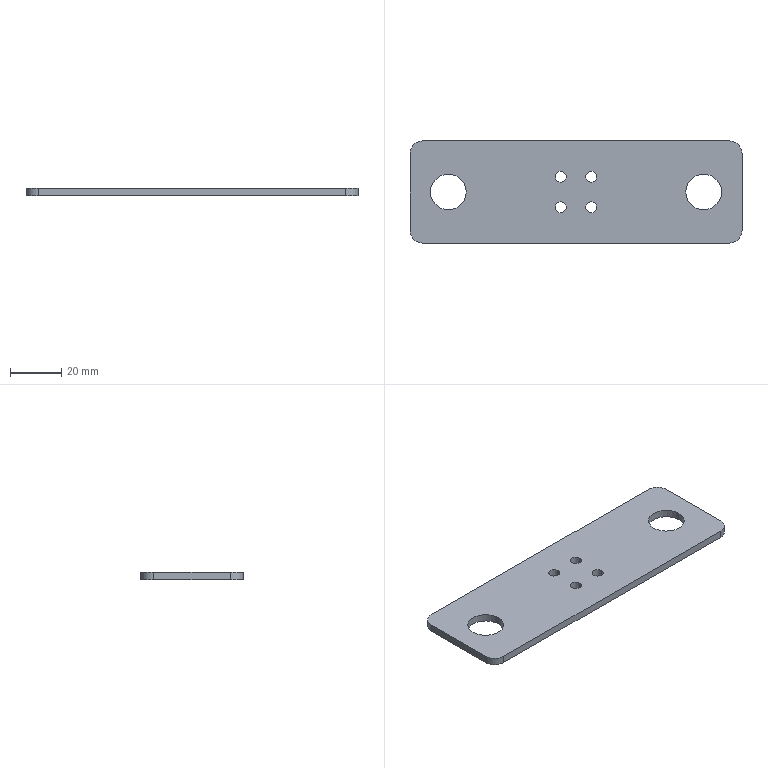Part | SolidWorks | features Extrusion 1, Fillet 1, ICE 1 | 1 solid | 22 faces | box 130 x 40 x 3 mm | volume 14438 mm3 | cylinder 16 | plane 6 | commonest cylinder face diameters 4.3 x8 10 x4 14 x4
STEP:
#1=CARTESIAN_POINT('',(-57.,0.,0.));
#2=VERTEX_POINT('',#1);
#3=CARTESIAN_POINT('',(-43.,0.,0.));
#4=VERTEX_POINT('',#3);
#5=CARTESIAN_POINT('',(-50.,0.,0.));
#6=DIRECTION('',(0.,0.,1.));
#7=DIRECTION('',(1.,0.,0.));
#8=AXIS2_PLACEMENT_3D('',#5,#6,#7);
#9=CIRCLE('',#8,7.);
#10=EDGE_CURVE('',#2,#4,#9,.T.);
#11=ORIENTED_EDGE('',*,*,#10,.F.);
#12=CARTESIAN_POINT('',(-57.,0.,3.));
#13=VERTEX_POINT('',#12);
#14=CARTESIAN_POINT('',(-57.,0.,0.));
#15=DIRECTION('',(0.,0.,1.));
#16=VECTOR('',#15,1000.);
#17=LINE('',#14,#16);
#18=EDGE_CURVE('',#2,#13,#17,.T.);
#19=ORIENTED_EDGE('',*,*,#18,.T.);
#20=CARTESIAN_POINT('',(-43.,0.,3.));
#21=VERTEX_POINT('',#20);
#22=CARTESIAN_POINT('',(-50.,0.,3.));
#23=DIRECTION('',(0.,0.,1.));
#24=DIRECTION('',(1.,0.,0.));
#25=AXIS2_PLACEMENT_3D('',#22,#23,#24);
#26=CIRCLE('',#25,7.);
#27=EDGE_CURVE('',#13,#21,#26,.T.);
#28=ORIENTED_EDGE('',*,*,#27,.T.);
#29=CARTESIAN_POINT('',(-43.,0.,0.));
#30=DIRECTION('',(0.,0.,1.));
#31=VECTOR('',#30,1000.);
#32=LINE('',#29,#31);
#33=EDGE_CURVE('',#4,#21,#32,.T.);
#34=ORIENTED_EDGE('',*,*,#33,.F.);
#35=EDGE_LOOP('',(#11,#19,#28,#34));
#36=FACE_OUTER_BOUND('',#35,.T.);
#37=CARTESIAN_POINT('',(-50.,0.,0.));
#38=DIRECTION('',(0.,0.,1.));
#39=DIRECTION('',(1.,0.,0.));
#40=AXIS2_PLACEMENT_3D('',#37,#38,#39);
#41=CYLINDRICAL_SURFACE('',#40,7.);
#42=ADVANCED_FACE('',(#36),#41,.F.);
#43=CARTESIAN_POINT('',(-8.15,-6.,0.));
#44=VERTEX_POINT('',#43);
#45=CARTESIAN_POINT('',(-3.85,-6.,0.));
#46=VERTEX_POINT('',#45);
#47=CARTESIAN_POINT('',(-6.,-6.,0.));
#48=DIRECTION('',(0.,0.,1.));
#49=DIRECTION('',(1.,0.,0.));
#50=AXIS2_PLACEMENT_3D('',#47,#48,#49);
#51=CIRCLE('',#50,2.15);
#52=EDGE_CURVE('',#44,#46,#51,.T.);
#53=ORIENTED_EDGE('',*,*,#52,.F.);
#54=CARTESIAN_POINT('',(-8.15,-6.,3.));
#55=VERTEX_POINT('',#54);
#56=CARTESIAN_POINT('',(-8.15,-6.,0.));
#57=DIRECTION('',(0.,0.,1.));
#58=VECTOR('',#57,1000.);
#59=LINE('',#56,#58);
#60=EDGE_CURVE('',#44,#55,#59,.T.);
#61=ORIENTED_EDGE('',*,*,#60,.T.);
#62=CARTESIAN_POINT('',(-3.85,-6.,3.));
#63=VERTEX_POINT('',#62);
#64=CARTESIAN_POINT('',(-6.,-6.,3.));
#65=DIRECTION('',(0.,0.,1.));
#66=DIRECTION('',(1.,0.,0.));
#67=AXIS2_PLACEMENT_3D('',#64,#65,#66);
#68=CIRCLE('',#67,2.15);
#69=EDGE_CURVE('',#55,#63,#68,.T.);
#70=ORIENTED_EDGE('',*,*,#69,.T.);
#71=CARTESIAN_POINT('',(-3.85,-6.,0.));
#72=DIRECTION('',(0.,0.,1.));
#73=VECTOR('',#72,1000.);
#74=LINE('',#71,#73);
#75=EDGE_CURVE('',#46,#63,#74,.T.);
#76=ORIENTED_EDGE('',*,*,#75,.F.);
#77=EDGE_LOOP('',(#53,#61,#70,#76));
#78=FACE_OUTER_BOUND('',#77,.T.);
#79=CARTESIAN_POINT('',(-6.,-6.,0.));
#80=DIRECTION('',(0.,0.,1.));
#81=DIRECTION('',(1.,0.,0.));
#82=AXIS2_PLACEMENT_3D('',#79,#80,#81);
#83=CYLINDRICAL_SURFACE('',#82,2.15);
#84=ADVANCED_FACE('',(#78),#83,.F.);
#85=CARTESIAN_POINT('',(43.,0.,0.));
#86=VERTEX_POINT('',#85);
#87=CARTESIAN_POINT('',(57.,0.,0.));
#88=VERTEX_POINT('',#87);
#89=CARTESIAN_POINT('',(50.,0.,0.));
#90=DIRECTION('',(0.,0.,1.));
#91=DIRECTION('',(1.,0.,0.));
#92=AXIS2_PLACEMENT_3D('',#89,#90,#91);
#93=CIRCLE('',#92,7.);
#94=EDGE_CURVE('',#86,#88,#93,.T.);
#95=ORIENTED_EDGE('',*,*,#94,.F.);
#96=CARTESIAN_POINT('',(43.,0.,3.));
#97=VERTEX_POINT('',#96);
#98=CARTESIAN_POINT('',(43.,0.,0.));
#99=DIRECTION('',(0.,0.,1.));
#100=VECTOR('',#99,1000.);
#101=LINE('',#98,#100);
#102=EDGE_CURVE('',#86,#97,#101,.T.);
#103=ORIENTED_EDGE('',*,*,#102,.T.);
#104=CARTESIAN_POINT('',(57.,0.,3.));
#105=VERTEX_POINT('',#104);
#106=CARTESIAN_POINT('',(50.,0.,3.));
#107=DIRECTION('',(0.,0.,1.));
#108=DIRECTION('',(1.,0.,0.));
#109=AXIS2_PLACEMENT_3D('',#106,#107,#108);
#110=CIRCLE('',#109,7.);
#111=EDGE_CURVE('',#97,#105,#110,.T.);
#112=ORIENTED_EDGE('',*,*,#111,.T.);
#113=CARTESIAN_POINT('',(57.,0.,0.));
#114=DIRECTION('',(0.,0.,1.));
#115=VECTOR('',#114,1000.);
#116=LINE('',#113,#115);
#117=EDGE_CURVE('',#88,#105,#116,.T.);
#118=ORIENTED_EDGE('',*,*,#117,.F.);
#119=EDGE_LOOP('',(#95,#103,#112,#118));
#120=FACE_OUTER_BOUND('',#119,.T.);
#121=CARTESIAN_POINT('',(50.,0.,0.));
#122=DIRECTION('',(0.,0.,1.));
#123=DIRECTION('',(1.,0.,0.));
#124=AXIS2_PLACEMENT_3D('',#121,#122,#123);
#125=CYLINDRICAL_SURFACE('',#124,7.);
#126=ADVANCED_FACE('',(#120),#125,.F.);
#127=CARTESIAN_POINT('',(-8.15,6.,0.));
#128=VERTEX_POINT('',#127);
#129=CARTESIAN_POINT('',(-3.85,6.,0.));
#130=VERTEX_POINT('',#129);
#131=CARTESIAN_POINT('',(-6.,6.,0.));
#132=DIRECTION('',(0.,0.,1.));
#133=DIRECTION('',(1.,0.,0.));
#134=AXIS2_PLACEMENT_3D('',#131,#132,#133);
#135=CIRCLE('',#134,2.15);
#136=EDGE_CURVE('',#128,#130,#135,.T.);
#137=ORIENTED_EDGE('',*,*,#136,.F.);
#138=CARTESIAN_POINT('',(-8.15,6.,3.));
#139=VERTEX_POINT('',#138);
#140=CARTESIAN_POINT('',(-8.15,6.,0.));
#141=DIRECTION('',(0.,0.,1.));
#142=VECTOR('',#141,1000.);
#143=LINE('',#140,#142);
#144=EDGE_CURVE('',#128,#139,#143,.T.);
#145=ORIENTED_EDGE('',*,*,#144,.T.);
#146=CARTESIAN_POINT('',(-3.85,6.,3.));
#147=VERTEX_POINT('',#146);
#148=CARTESIAN_POINT('',(-6.,6.,3.));
#149=DIRECTION('',(0.,0.,1.));
#150=DIRECTION('',(1.,0.,0.));
#151=AXIS2_PLACEMENT_3D('',#148,#149,#150);
#152=CIRCLE('',#151,2.15);
#153=EDGE_CURVE('',#139,#147,#152,.T.);
#154=ORIENTED_EDGE('',*,*,#153,.T.);
#155=CARTESIAN_POINT('',(-3.85,6.,0.));
#156=DIRECTION('',(0.,0.,1.));
#157=VECTOR('',#156,1000.);
#158=LINE('',#155,#157);
#159=EDGE_CURVE('',#130,#147,#158,.T.);
#160=ORIENTED_EDGE('',*,*,#159,.F.);
#161=EDGE_LOOP('',(#137,#145,#154,#160));
#162=FACE_OUTER_BOUND('',#161,.T.);
#163=CARTESIAN_POINT('',(-6.,6.,0.));
#164=DIRECTION('',(0.,0.,1.));
#165=DIRECTION('',(1.,0.,0.));
#166=AXIS2_PLACEMENT_3D('',#163,#164,#165);
#167=CYLINDRICAL_SURFACE('',#166,2.15);
#168=ADVANCED_FACE('',(#162),#167,.F.);
#169=CARTESIAN_POINT('',(3.85,6.,0.));
#170=VERTEX_POINT('',#169);
#171=CARTESIAN_POINT('',(8.15,6.,0.));
#172=VERTEX_POINT('',#171);
#173=CARTESIAN_POINT('',(6.,6.,0.));
#174=DIRECTION('',(0.,0.,1.));
#175=DIRECTION('',(1.,0.,0.));
#176=AXIS2_PLACEMENT_3D('',#173,#174,#175);
#177=CIRCLE('',#176,2.15);
#178=EDGE_CURVE('',#170,#172,#177,.T.);
#179=ORIENTED_EDGE('',*,*,#178,.F.);
#180=CARTESIAN_POINT('',(3.85,6.,3.));
#181=VERTEX_POINT('',#180);
#182=CARTESIAN_POINT('',(3.85,6.,0.));
#183=DIRECTION('',(0.,0.,1.));
#184=VECTOR('',#183,1000.);
#185=LINE('',#182,#184);
#186=EDGE_CURVE('',#170,#181,#185,.T.);
#187=ORIENTED_EDGE('',*,*,#186,.T.);
#188=CARTESIAN_POINT('',(8.15,6.,3.));
#189=VERTEX_POINT('',#188);
#190=CARTESIAN_POINT('',(6.,6.,3.));
#191=DIRECTION('',(0.,0.,1.));
#192=DIRECTION('',(1.,0.,0.));
#193=AXIS2_PLACEMENT_3D('',#190,#191,#192);
#194=CIRCLE('',#193,2.15);
#195=EDGE_CURVE('',#181,#189,#194,.T.);
#196=ORIENTED_EDGE('',*,*,#195,.T.);
#197=CARTESIAN_POINT('',(8.15,6.,0.));
#198=DIRECTION('',(0.,0.,1.));
#199=VECTOR('',#198,1000.);
#200=LINE('',#197,#199);
#201=EDGE_CURVE('',#172,#189,#200,.T.);
#202=ORIENTED_EDGE('',*,*,#201,.F.);
#203=EDGE_LOOP('',(#179,#187,#196,#202));
#204=FACE_OUTER_BOUND('',#203,.T.);
#205=CARTESIAN_POINT('',(6.,6.,0.));
#206=DIRECTION('',(0.,0.,1.));
#207=DIRECTION('',(1.,0.,0.));
#208=AXIS2_PLACEMENT_3D('',#205,#206,#207);
#209=CYLINDRICAL_SURFACE('',#208,2.15);
#210=ADVANCED_FACE('',(#204),#209,.F.);
#211=CARTESIAN_POINT('',(3.85,-6.,0.));
#212=VERTEX_POINT('',#211);
#213=CARTESIAN_POINT('',(8.15,-6.,0.));
#214=VERTEX_POINT('',#213);
#215=CARTESIAN_POINT('',(6.,-6.,0.));
#216=DIRECTION('',(0.,0.,1.));
#217=DIRECTION('',(1.,0.,0.));
#218=AXIS2_PLACEMENT_3D('',#215,#216,#217);
#219=CIRCLE('',#218,2.15);
#220=EDGE_CURVE('',#212,#214,#219,.T.);
#221=ORIENTED_EDGE('',*,*,#220,.F.);
#222=CARTESIAN_POINT('',(3.85,-6.,3.));
#223=VERTEX_POINT('',#222);
#224=CARTESIAN_POINT('',(3.85,-6.,0.));
#225=DIRECTION('',(0.,0.,1.));
#226=VECTOR('',#225,1000.);
#227=LINE('',#224,#226);
#228=EDGE_CURVE('',#212,#223,#227,.T.);
#229=ORIENTED_EDGE('',*,*,#228,.T.);
#230=CARTESIAN_POINT('',(8.15,-6.,3.));
#231=VERTEX_POINT('',#230);
#232=CARTESIAN_POINT('',(6.,-6.,3.));
#233=DIRECTION('',(0.,0.,1.));
#234=DIRECTION('',(1.,0.,0.));
#235=AXIS2_PLACEMENT_3D('',#232,#233,#234);
#236=CIRCLE('',#235,2.15);
#237=EDGE_CURVE('',#223,#231,#236,.T.);
#238=ORIENTED_EDGE('',*,*,#237,.T.);
#239=CARTESIAN_POINT('',(8.15,-6.,0.));
#240=DIRECTION('',(0.,0.,1.));
#241=VECTOR('',#240,1000.);
#242=LINE('',#239,#241);
#243=EDGE_CURVE('',#214,#231,#242,.T.);
#244=ORIENTED_EDGE('',*,*,#243,.F.);
#245=EDGE_LOOP('',(#221,#229,#238,#244));
#246=FACE_OUTER_BOUND('',#245,.T.);
#247=CARTESIAN_POINT('',(6.,-6.,0.));
#248=DIRECTION('',(0.,0.,1.));
#249=DIRECTION('',(1.,0.,0.));
#250=AXIS2_PLACEMENT_3D('',#247,#248,#249);
#251=CYLINDRICAL_SURFACE('',#250,2.15);
#252=ADVANCED_FACE('',(#246),#251,.F.);
#253=CARTESIAN_POINT('',(65.,-15.,0.));
#254=VERTEX_POINT('',#253);
#255=CARTESIAN_POINT('',(65.,15.,0.));
#256=VERTEX_POINT('',#255);
#257=CARTESIAN_POINT('',(65.,20.,0.));
#258=DIRECTION('',(0.,1.,0.));
#259=VECTOR('',#258,1000.);
#260=LINE('',#257,#259);
#261=EDGE_CURVE('',#254,#256,#260,.T.);
#262=ORIENTED_EDGE('',*,*,#261,.T.);
#263=CARTESIAN_POINT('',(65.,15.,3.));
#264=VERTEX_POINT('',#263);
#265=CARTESIAN_POINT('',(65.,15.,3.));
#266=DIRECTION('',(0.,0.,1.));
#267=VECTOR('',#266,1000.);
#268=LINE('',#265,#267);
#269=EDGE_CURVE('',#256,#264,#268,.T.);
#270=ORIENTED_EDGE('',*,*,#269,.T.);
#271=CARTESIAN_POINT('',(65.,-15.,3.));
#272=VERTEX_POINT('',#271);
#273=CARTESIAN_POINT('',(65.,20.,3.));
#274=DIRECTION('',(0.,1.,0.));
#275=VECTOR('',#274,1000.);
#276=LINE('',#273,#275);
#277=EDGE_CURVE('',#272,#264,#276,.T.);
#278=ORIENTED_EDGE('',*,*,#277,.F.);
#279=CARTESIAN_POINT('',(65.,-15.,3.));
#280=DIRECTION('',(0.,0.,-1.));
#281=VECTOR('',#280,1000.);
#282=LINE('',#279,#281);
#283=EDGE_CURVE('',#272,#254,#282,.T.);
#284=ORIENTED_EDGE('',*,*,#283,.T.);
#285=EDGE_LOOP('',(#262,#270,#278,#284));
#286=FACE_OUTER_BOUND('',#285,.T.);
#287=CARTESIAN_POINT('',(65.,20.,3.));
#288=DIRECTION('',(-1.,0.,0.));
#289=DIRECTION('',(0.,0.,1.));
#290=AXIS2_PLACEMENT_3D('',#287,#288,#289);
#291=PLANE('',#290);
#292=ADVANCED_FACE('',(#286),#291,.F.);
#293=CARTESIAN_POINT('',(60.,20.,3.));
#294=VERTEX_POINT('',#293);
#295=CARTESIAN_POINT('',(-60.,20.,3.));
#296=VERTEX_POINT('',#295);
#297=CARTESIAN_POINT('',(-65.,20.,3.));
#298=DIRECTION('',(-1.,0.,0.));
#299=VECTOR('',#298,1000.);
#300=LINE('',#297,#299);
#301=EDGE_CURVE('',#294,#296,#300,.T.);
#302=ORIENTED_EDGE('',*,*,#301,.F.);
#303=CARTESIAN_POINT('',(60.,20.,0.));
#304=VERTEX_POINT('',#303);
#305=CARTESIAN_POINT('',(60.,20.,3.));
#306=DIRECTION('',(0.,0.,-1.));
#307=VECTOR('',#306,1000.);
#308=LINE('',#305,#307);
#309=EDGE_CURVE('',#294,#304,#308,.T.);
#310=ORIENTED_EDGE('',*,*,#309,.T.);
#311=CARTESIAN_POINT('',(-60.,20.,0.));
#312=VERTEX_POINT('',#311);
#313=CARTESIAN_POINT('',(-65.,20.,0.));
#314=DIRECTION('',(-1.,0.,0.));
#315=VECTOR('',#314,1000.);
#316=LINE('',#313,#315);
#317=EDGE_CURVE('',#304,#312,#316,.T.);
#318=ORIENTED_EDGE('',*,*,#317,.T.);
#319=CARTESIAN_POINT('',(-60.,20.,3.));
#320=DIRECTION('',(0.,0.,1.));
#321=VECTOR('',#320,1000.);
#322=LINE('',#319,#321);
#323=EDGE_CURVE('',#312,#296,#322,.T.);
#324=ORIENTED_EDGE('',*,*,#323,.T.);
#325=EDGE_LOOP('',(#302,#310,#318,#324));
#326=FACE_OUTER_BOUND('',#325,.T.);
#327=CARTESIAN_POINT('',(-65.,20.,3.));
#328=DIRECTION('',(0.,-1.,0.));
#329=DIRECTION('',(0.,0.,-1.));
#330=AXIS2_PLACEMENT_3D('',#327,#328,#329);
#331=PLANE('',#330);
#332=ADVANCED_FACE('',(#326),#331,.F.);
#333=CARTESIAN_POINT('',(-65.,15.,3.));
#334=VERTEX_POINT('',#333);
#335=CARTESIAN_POINT('',(-65.,-15.,3.));
#336=VERTEX_POINT('',#335);
#337=CARTESIAN_POINT('',(-65.,20.,3.));
#338=DIRECTION('',(0.,-1.,0.));
#339=VECTOR('',#338,1000.);
#340=LINE('',#337,#339);
#341=EDGE_CURVE('',#334,#336,#340,.T.);
#342=ORIENTED_EDGE('',*,*,#341,.F.);
#343=CARTESIAN_POINT('',(-65.,15.,0.));
#344=VERTEX_POINT('',#343);
#345=CARTESIAN_POINT('',(-65.,15.,3.));
#346=DIRECTION('',(0.,0.,-1.));
#347=VECTOR('',#346,1000.);
#348=LINE('',#345,#347);
#349=EDGE_CURVE('',#334,#344,#348,.T.);
#350=ORIENTED_EDGE('',*,*,#349,.T.);
#351=CARTESIAN_POINT('',(-65.,-15.,0.));
#352=VERTEX_POINT('',#351);
#353=CARTESIAN_POINT('',(-65.,20.,0.));
#354=DIRECTION('',(0.,-1.,0.));
#355=VECTOR('',#354,1000.);
#356=LINE('',#353,#355);
#357=EDGE_CURVE('',#344,#352,#356,.T.);
#358=ORIENTED_EDGE('',*,*,#357,.T.);
#359=CARTESIAN_POINT('',(-65.,-15.,3.));
#360=DIRECTION('',(0.,0.,1.));
#361=VECTOR('',#360,1000.);
#362=LINE('',#359,#361);
#363=EDGE_CURVE('',#352,#336,#362,.T.);
#364=ORIENTED_EDGE('',*,*,#363,.T.);
#365=EDGE_LOOP('',(#342,#350,#358,#364));
#366=FACE_OUTER_BOUND('',#365,.T.);
#367=CARTESIAN_POINT('',(-65.,20.,3.));
#368=DIRECTION('',(1.,0.,0.));
#369=DIRECTION('',(0.,0.,-1.));
#370=AXIS2_PLACEMENT_3D('',#367,#368,#369);
#371=PLANE('',#370);
#372=ADVANCED_FACE('',(#366),#371,.F.);
#373=CARTESIAN_POINT('',(-60.,-20.,0.));
#374=VERTEX_POINT('',#373);
#375=CARTESIAN_POINT('',(60.,-20.,0.));
#376=VERTEX_POINT('',#375);
#377=CARTESIAN_POINT('',(-65.,-20.,0.));
#378=DIRECTION('',(1.,0.,0.));
#379=VECTOR('',#378,1000.);
#380=LINE('',#377,#379);
#381=EDGE_CURVE('',#374,#376,#380,.T.);
#382=ORIENTED_EDGE('',*,*,#381,.T.);
#383=CARTESIAN_POINT('',(60.,-20.,3.));
#384=VERTEX_POINT('',#383);
#385=CARTESIAN_POINT('',(60.,-20.,3.));
#386=DIRECTION('',(0.,0.,1.));
#387=VECTOR('',#386,1000.);
#388=LINE('',#385,#387);
#389=EDGE_CURVE('',#376,#384,#388,.T.);
#390=ORIENTED_EDGE('',*,*,#389,.T.);
#391=CARTESIAN_POINT('',(-60.,-20.,3.));
#392=VERTEX_POINT('',#391);
#393=CARTESIAN_POINT('',(-65.,-20.,3.));
#394=DIRECTION('',(1.,0.,0.));
#395=VECTOR('',#394,1000.);
#396=LINE('',#393,#395);
#397=EDGE_CURVE('',#392,#384,#396,.T.);
#398=ORIENTED_EDGE('',*,*,#397,.F.);
#399=CARTESIAN_POINT('',(-60.,-20.,3.));
#400=DIRECTION('',(0.,0.,-1.));
#401=VECTOR('',#400,1000.);
#402=LINE('',#399,#401);
#403=EDGE_CURVE('',#392,#374,#402,.T.);
#404=ORIENTED_EDGE('',*,*,#403,.T.);
#405=EDGE_LOOP('',(#382,#390,#398,#404));
#406=FACE_OUTER_BOUND('',#405,.T.);
#407=CARTESIAN_POINT('',(-65.,-20.,3.));
#408=DIRECTION('',(0.,1.,0.));
#409=DIRECTION('',(0.,0.,1.));
#410=AXIS2_PLACEMENT_3D('',#407,#408,#409);
#411=PLANE('',#410);
#412=ADVANCED_FACE('',(#406),#411,.F.);
#413=CARTESIAN_POINT('',(-50.,0.,3.));
#414=DIRECTION('',(0.,0.,1.));
#415=DIRECTION('',(1.,0.,0.));
#416=AXIS2_PLACEMENT_3D('',#413,#414,#415);
#417=CIRCLE('',#416,7.);
#418=EDGE_CURVE('',#21,#13,#417,.T.);
#419=ORIENTED_EDGE('',*,*,#418,.F.);
#420=ORIENTED_EDGE('',*,*,#27,.F.);
#421=EDGE_LOOP('',(#419,#420));
#422=FACE_BOUND('',#421,.T.);
#423=CARTESIAN_POINT('',(-6.,-6.,3.));
#424=DIRECTION('',(0.,0.,1.));
#425=DIRECTION('',(1.,0.,0.));
#426=AXIS2_PLACEMENT_3D('',#423,#424,#425);
#427=CIRCLE('',#426,2.15);
#428=EDGE_CURVE('',#63,#55,#427,.T.);
#429=ORIENTED_EDGE('',*,*,#428,.F.);
#430=ORIENTED_EDGE('',*,*,#69,.F.);
#431=EDGE_LOOP('',(#429,#430));
#432=FACE_BOUND('',#431,.T.);
#433=CARTESIAN_POINT('',(50.,0.,3.));
#434=DIRECTION('',(0.,0.,1.));
#435=DIRECTION('',(1.,0.,0.));
#436=AXIS2_PLACEMENT_3D('',#433,#434,#435);
#437=CIRCLE('',#436,7.);
#438=EDGE_CURVE('',#105,#97,#437,.T.);
#439=ORIENTED_EDGE('',*,*,#438,.F.);
#440=ORIENTED_EDGE('',*,*,#111,.F.);
#441=EDGE_LOOP('',(#439,#440));
#442=FACE_BOUND('',#441,.T.);
#443=CARTESIAN_POINT('',(-6.,6.,3.));
#444=DIRECTION('',(0.,0.,1.));
#445=DIRECTION('',(1.,0.,0.));
#446=AXIS2_PLACEMENT_3D('',#443,#444,#445);
#447=CIRCLE('',#446,2.15);
#448=EDGE_CURVE('',#147,#139,#447,.T.);
#449=ORIENTED_EDGE('',*,*,#448,.F.);
#450=ORIENTED_EDGE('',*,*,#153,.F.);
#451=EDGE_LOOP('',(#449,#450));
#452=FACE_BOUND('',#451,.T.);
#453=CARTESIAN_POINT('',(6.,6.,3.));
#454=DIRECTION('',(0.,0.,1.));
#455=DIRECTION('',(1.,0.,0.));
#456=AXIS2_PLACEMENT_3D('',#453,#454,#455);
#457=CIRCLE('',#456,2.15);
#458=EDGE_CURVE('',#189,#181,#457,.T.);
#459=ORIENTED_EDGE('',*,*,#458,.F.);
#460=ORIENTED_EDGE('',*,*,#195,.F.);
#461=EDGE_LOOP('',(#459,#460));
#462=FACE_BOUND('',#461,.T.);
#463=CARTESIAN_POINT('',(6.,-6.,3.));
#464=DIRECTION('',(0.,0.,1.));
#465=DIRECTION('',(1.,0.,0.));
#466=AXIS2_PLACEMENT_3D('',#463,#464,#465);
#467=CIRCLE('',#466,2.15);
#468=EDGE_CURVE('',#231,#223,#467,.T.);
#469=ORIENTED_EDGE('',*,*,#468,.F.);
#470=ORIENTED_EDGE('',*,*,#237,.F.);
#471=EDGE_LOOP('',(#469,#470));
#472=FACE_BOUND('',#471,.T.);
#473=ORIENTED_EDGE('',*,*,#277,.T.);
#474=CARTESIAN_POINT('',(60.,15.,3.));
#475=DIRECTION('',(0.,0.,1.));
#476=DIRECTION('',(1.,0.,0.));
#477=AXIS2_PLACEMENT_3D('',#474,#475,#476);
#478=CIRCLE('',#477,5.);
#479=EDGE_CURVE('',#264,#294,#478,.T.);
#480=ORIENTED_EDGE('',*,*,#479,.T.);
#481=ORIENTED_EDGE('',*,*,#301,.T.);
#482=CARTESIAN_POINT('',(-60.,15.,3.));
#483=DIRECTION('',(0.,0.,1.));
#484=DIRECTION('',(1.,0.,0.));
#485=AXIS2_PLACEMENT_3D('',#482,#483,#484);
#486=CIRCLE('',#485,5.);
#487=EDGE_CURVE('',#296,#334,#486,.T.);
#488=ORIENTED_EDGE('',*,*,#487,.T.);
#489=ORIENTED_EDGE('',*,*,#341,.T.);
#490=CARTESIAN_POINT('',(-60.,-15.,3.));
#491=DIRECTION('',(0.,0.,1.));
#492=DIRECTION('',(1.,0.,0.));
#493=AXIS2_PLACEMENT_3D('',#490,#491,#492);
#494=CIRCLE('',#493,5.);
#495=EDGE_CURVE('',#336,#392,#494,.T.);
#496=ORIENTED_EDGE('',*,*,#495,.T.);
#497=ORIENTED_EDGE('',*,*,#397,.T.);
#498=CARTESIAN_POINT('',(60.,-15.,3.));
#499=DIRECTION('',(0.,0.,1.));
#500=DIRECTION('',(1.,0.,0.));
#501=AXIS2_PLACEMENT_3D('',#498,#499,#500);
#502=CIRCLE('',#501,5.);
#503=EDGE_CURVE('',#384,#272,#502,.T.);
#504=ORIENTED_EDGE('',*,*,#503,.T.);
#505=EDGE_LOOP('',(#473,#480,#481,#488,#489,#496,#497,#504));
#506=FACE_OUTER_BOUND('',#505,.T.);
#507=CARTESIAN_POINT('',(0.,0.,3.));
#508=DIRECTION('',(0.,0.,1.));
#509=DIRECTION('',(1.,0.,0.));
#510=AXIS2_PLACEMENT_3D('',#507,#508,#509);
#511=PLANE('',#510);
#512=ADVANCED_FACE('',(#422,#432,#442,#452,#462,#472,#506),#511,.T.);
#513=CARTESIAN_POINT('',(-50.,0.,0.));
#514=DIRECTION('',(0.,0.,1.));
#515=DIRECTION('',(1.,0.,0.));
#516=AXIS2_PLACEMENT_3D('',#513,#514,#515);
#517=CIRCLE('',#516,7.);
#518=EDGE_CURVE('',#4,#2,#517,.T.);
#519=ORIENTED_EDGE('',*,*,#518,.T.);
#520=ORIENTED_EDGE('',*,*,#10,.T.);
#521=EDGE_LOOP('',(#519,#520));
#522=FACE_BOUND('',#521,.T.);
#523=CARTESIAN_POINT('',(-6.,-6.,0.));
#524=DIRECTION('',(0.,0.,1.));
#525=DIRECTION('',(1.,0.,0.));
#526=AXIS2_PLACEMENT_3D('',#523,#524,#525);
#527=CIRCLE('',#526,2.15);
#528=EDGE_CURVE('',#46,#44,#527,.T.);
#529=ORIENTED_EDGE('',*,*,#528,.T.);
#530=ORIENTED_EDGE('',*,*,#52,.T.);
#531=EDGE_LOOP('',(#529,#530));
#532=FACE_BOUND('',#531,.T.);
#533=CARTESIAN_POINT('',(50.,0.,0.));
#534=DIRECTION('',(0.,0.,1.));
#535=DIRECTION('',(1.,0.,0.));
#536=AXIS2_PLACEMENT_3D('',#533,#534,#535);
#537=CIRCLE('',#536,7.);
#538=EDGE_CURVE('',#88,#86,#537,.T.);
#539=ORIENTED_EDGE('',*,*,#538,.T.);
#540=ORIENTED_EDGE('',*,*,#94,.T.);
#541=EDGE_LOOP('',(#539,#540));
#542=FACE_BOUND('',#541,.T.);
#543=CARTESIAN_POINT('',(-6.,6.,0.));
#544=DIRECTION('',(0.,0.,1.));
#545=DIRECTION('',(1.,0.,0.));
#546=AXIS2_PLACEMENT_3D('',#543,#544,#545);
#547=CIRCLE('',#546,2.15);
#548=EDGE_CURVE('',#130,#128,#547,.T.);
#549=ORIENTED_EDGE('',*,*,#548,.T.);
#550=ORIENTED_EDGE('',*,*,#136,.T.);
#551=EDGE_LOOP('',(#549,#550));
#552=FACE_BOUND('',#551,.T.);
#553=CARTESIAN_POINT('',(6.,6.,0.));
#554=DIRECTION('',(0.,0.,1.));
#555=DIRECTION('',(1.,0.,0.));
#556=AXIS2_PLACEMENT_3D('',#553,#554,#555);
#557=CIRCLE('',#556,2.15);
#558=EDGE_CURVE('',#172,#170,#557,.T.);
#559=ORIENTED_EDGE('',*,*,#558,.T.);
#560=ORIENTED_EDGE('',*,*,#178,.T.);
#561=EDGE_LOOP('',(#559,#560));
#562=FACE_BOUND('',#561,.T.);
#563=CARTESIAN_POINT('',(6.,-6.,0.));
#564=DIRECTION('',(0.,0.,1.));
#565=DIRECTION('',(1.,0.,0.));
#566=AXIS2_PLACEMENT_3D('',#563,#564,#565);
#567=CIRCLE('',#566,2.15);
#568=EDGE_CURVE('',#214,#212,#567,.T.);
#569=ORIENTED_EDGE('',*,*,#568,.T.);
#570=ORIENTED_EDGE('',*,*,#220,.T.);
#571=EDGE_LOOP('',(#569,#570));
#572=FACE_BOUND('',#571,.T.);
#573=ORIENTED_EDGE('',*,*,#317,.F.);
#574=CARTESIAN_POINT('',(60.,15.,0.));
#575=DIRECTION('',(0.,0.,-1.));
#576=DIRECTION('',(1.,0.,0.));
#577=AXIS2_PLACEMENT_3D('',#574,#575,#576);
#578=CIRCLE('',#577,5.);
#579=EDGE_CURVE('',#304,#256,#578,.T.);
#580=ORIENTED_EDGE('',*,*,#579,.T.);
#581=ORIENTED_EDGE('',*,*,#261,.F.);
#582=CARTESIAN_POINT('',(60.,-15.,0.));
#583=DIRECTION('',(0.,0.,-1.));
#584=DIRECTION('',(1.,0.,0.));
#585=AXIS2_PLACEMENT_3D('',#582,#583,#584);
#586=CIRCLE('',#585,5.);
#587=EDGE_CURVE('',#254,#376,#586,.T.);
#588=ORIENTED_EDGE('',*,*,#587,.T.);
#589=ORIENTED_EDGE('',*,*,#381,.F.);
#590=CARTESIAN_POINT('',(-60.,-15.,0.));
#591=DIRECTION('',(0.,0.,-1.));
#592=DIRECTION('',(1.,0.,0.));
#593=AXIS2_PLACEMENT_3D('',#590,#591,#592);
#594=CIRCLE('',#593,5.);
#595=EDGE_CURVE('',#374,#352,#594,.T.);
#596=ORIENTED_EDGE('',*,*,#595,.T.);
#597=ORIENTED_EDGE('',*,*,#357,.F.);
#598=CARTESIAN_POINT('',(-60.,15.,0.));
#599=DIRECTION('',(0.,0.,-1.));
#600=DIRECTION('',(1.,0.,0.));
#601=AXIS2_PLACEMENT_3D('',#598,#599,#600);
#602=CIRCLE('',#601,5.);
#603=EDGE_CURVE('',#344,#312,#602,.T.);
#604=ORIENTED_EDGE('',*,*,#603,.T.);
#605=EDGE_LOOP('',(#573,#580,#581,#588,#589,#596,#597,#604));
#606=FACE_OUTER_BOUND('',#605,.T.);
#607=CARTESIAN_POINT('',(0.,0.,0.));
#608=DIRECTION('',(0.,0.,1.));
#609=DIRECTION('',(1.,0.,0.));
#610=AXIS2_PLACEMENT_3D('',#607,#608,#609);
#611=PLANE('',#610);
#612=ADVANCED_FACE('',(#522,#532,#542,#552,#562,#572,#606),#611,.F.);
#613=ORIENTED_EDGE('',*,*,#228,.F.);
#614=ORIENTED_EDGE('',*,*,#568,.F.);
#615=ORIENTED_EDGE('',*,*,#243,.T.);
#616=ORIENTED_EDGE('',*,*,#468,.T.);
#617=EDGE_LOOP('',(#613,#614,#615,#616));
#618=FACE_OUTER_BOUND('',#617,.T.);
#619=CARTESIAN_POINT('',(6.,-6.,0.));
#620=DIRECTION('',(0.,0.,1.));
#621=DIRECTION('',(1.,0.,0.));
#622=AXIS2_PLACEMENT_3D('',#619,#620,#621);
#623=CYLINDRICAL_SURFACE('',#622,2.15);
#624=ADVANCED_FACE('',(#618),#623,.F.);
#625=ORIENTED_EDGE('',*,*,#186,.F.);
#626=ORIENTED_EDGE('',*,*,#558,.F.);
#627=ORIENTED_EDGE('',*,*,#201,.T.);
#628=ORIENTED_EDGE('',*,*,#458,.T.);
#629=EDGE_LOOP('',(#625,#626,#627,#628));
#630=FACE_OUTER_BOUND('',#629,.T.);
#631=CARTESIAN_POINT('',(6.,6.,0.));
#632=DIRECTION('',(0.,0.,1.));
#633=DIRECTION('',(1.,0.,0.));
#634=AXIS2_PLACEMENT_3D('',#631,#632,#633);
#635=CYLINDRICAL_SURFACE('',#634,2.15);
#636=ADVANCED_FACE('',(#630),#635,.F.);
#637=ORIENTED_EDGE('',*,*,#144,.F.);
#638=ORIENTED_EDGE('',*,*,#548,.F.);
#639=ORIENTED_EDGE('',*,*,#159,.T.);
#640=ORIENTED_EDGE('',*,*,#448,.T.);
#641=EDGE_LOOP('',(#637,#638,#639,#640));
#642=FACE_OUTER_BOUND('',#641,.T.);
#643=CARTESIAN_POINT('',(-6.,6.,0.));
#644=DIRECTION('',(0.,0.,1.));
#645=DIRECTION('',(1.,0.,0.));
#646=AXIS2_PLACEMENT_3D('',#643,#644,#645);
#647=CYLINDRICAL_SURFACE('',#646,2.15);
#648=ADVANCED_FACE('',(#642),#647,.F.);
#649=ORIENTED_EDGE('',*,*,#102,.F.);
#650=ORIENTED_EDGE('',*,*,#538,.F.);
#651=ORIENTED_EDGE('',*,*,#117,.T.);
#652=ORIENTED_EDGE('',*,*,#438,.T.);
#653=EDGE_LOOP('',(#649,#650,#651,#652));
#654=FACE_OUTER_BOUND('',#653,.T.);
#655=CARTESIAN_POINT('',(50.,0.,0.));
#656=DIRECTION('',(0.,0.,1.));
#657=DIRECTION('',(1.,0.,0.));
#658=AXIS2_PLACEMENT_3D('',#655,#656,#657);
#659=CYLINDRICAL_SURFACE('',#658,7.);
#660=ADVANCED_FACE('',(#654),#659,.F.);
#661=ORIENTED_EDGE('',*,*,#60,.F.);
#662=ORIENTED_EDGE('',*,*,#528,.F.);
#663=ORIENTED_EDGE('',*,*,#75,.T.);
#664=ORIENTED_EDGE('',*,*,#428,.T.);
#665=EDGE_LOOP('',(#661,#662,#663,#664));
#666=FACE_OUTER_BOUND('',#665,.T.);
#667=CARTESIAN_POINT('',(-6.,-6.,0.));
#668=DIRECTION('',(0.,0.,1.));
#669=DIRECTION('',(1.,0.,0.));
#670=AXIS2_PLACEMENT_3D('',#667,#668,#669);
#671=CYLINDRICAL_SURFACE('',#670,2.15);
#672=ADVANCED_FACE('',(#666),#671,.F.);
#673=ORIENTED_EDGE('',*,*,#18,.F.);
#674=ORIENTED_EDGE('',*,*,#518,.F.);
#675=ORIENTED_EDGE('',*,*,#33,.T.);
#676=ORIENTED_EDGE('',*,*,#418,.T.);
#677=EDGE_LOOP('',(#673,#674,#675,#676));
#678=FACE_OUTER_BOUND('',#677,.T.);
#679=CARTESIAN_POINT('',(-50.,0.,0.));
#680=DIRECTION('',(0.,0.,1.));
#681=DIRECTION('',(1.,0.,0.));
#682=AXIS2_PLACEMENT_3D('',#679,#680,#681);
#683=CYLINDRICAL_SURFACE('',#682,7.);
#684=ADVANCED_FACE('',(#678),#683,.F.);
#685=ORIENTED_EDGE('',*,*,#479,.F.);
#686=ORIENTED_EDGE('',*,*,#269,.F.);
#687=ORIENTED_EDGE('',*,*,#579,.F.);
#688=ORIENTED_EDGE('',*,*,#309,.F.);
#689=EDGE_LOOP('',(#685,#686,#687,#688));
#690=FACE_OUTER_BOUND('',#689,.T.);
#691=CARTESIAN_POINT('',(60.,15.,3.));
#692=DIRECTION('',(0.,0.,-1.));
#693=DIRECTION('',(-1.,0.,0.));
#694=AXIS2_PLACEMENT_3D('',#691,#692,#693);
#695=CYLINDRICAL_SURFACE('',#694,5.);
#696=ADVANCED_FACE('',(#690),#695,.T.);
#697=ORIENTED_EDGE('',*,*,#503,.F.);
#698=ORIENTED_EDGE('',*,*,#389,.F.);
#699=ORIENTED_EDGE('',*,*,#587,.F.);
#700=ORIENTED_EDGE('',*,*,#283,.F.);
#701=EDGE_LOOP('',(#697,#698,#699,#700));
#702=FACE_OUTER_BOUND('',#701,.T.);
#703=CARTESIAN_POINT('',(60.,-15.,3.));
#704=DIRECTION('',(0.,0.,-1.));
#705=DIRECTION('',(-1.,0.,0.));
#706=AXIS2_PLACEMENT_3D('',#703,#704,#705);
#707=CYLINDRICAL_SURFACE('',#706,5.);
#708=ADVANCED_FACE('',(#702),#707,.T.);
#709=ORIENTED_EDGE('',*,*,#487,.F.);
#710=ORIENTED_EDGE('',*,*,#323,.F.);
#711=ORIENTED_EDGE('',*,*,#603,.F.);
#712=ORIENTED_EDGE('',*,*,#349,.F.);
#713=EDGE_LOOP('',(#709,#710,#711,#712));
#714=FACE_OUTER_BOUND('',#713,.T.);
#715=CARTESIAN_POINT('',(-60.,15.,3.));
#716=DIRECTION('',(0.,0.,-1.));
#717=DIRECTION('',(-1.,0.,0.));
#718=AXIS2_PLACEMENT_3D('',#715,#716,#717);
#719=CYLINDRICAL_SURFACE('',#718,5.);
#720=ADVANCED_FACE('',(#714),#719,.T.);
#721=ORIENTED_EDGE('',*,*,#495,.F.);
#722=ORIENTED_EDGE('',*,*,#363,.F.);
#723=ORIENTED_EDGE('',*,*,#595,.F.);
#724=ORIENTED_EDGE('',*,*,#403,.F.);
#725=EDGE_LOOP('',(#721,#722,#723,#724));
#726=FACE_OUTER_BOUND('',#725,.T.);
#727=CARTESIAN_POINT('',(-60.,-15.,3.));
#728=DIRECTION('',(0.,0.,-1.));
#729=DIRECTION('',(-1.,0.,0.));
#730=AXIS2_PLACEMENT_3D('',#727,#728,#729);
#731=CYLINDRICAL_SURFACE('',#730,5.);
#732=ADVANCED_FACE('',(#726),#731,.T.);
#733=CLOSED_SHELL('',(#42,#84,#126,#168,#210,#252,#292,#332,#372,#412,#512,#612,#624,#636,#648,#660,#672,#684,#696,#708,#720,#732));
#734=MANIFOLD_SOLID_BREP('',#733);
#735=CARTESIAN_POINT('',(0.,0.,0.));
#736=DIRECTION('',(0.,0.,1.));
#737=DIRECTION('',(1.,0.,0.));
#738=AXIS2_PLACEMENT_3D('',#735,#736,#737);
#739=(LENGTH_UNIT()NAMED_UNIT(*)SI_UNIT(.MILLI.,.METRE.));
#740=UNCERTAINTY_MEASURE_WITH_UNIT(LENGTH_MEASURE(0.00001),#739,'','');
#741=(NAMED_UNIT(*)PLANE_ANGLE_UNIT()SI_UNIT($,.RADIAN.));
#742=(NAMED_UNIT(*)SI_UNIT($,.STERADIAN.)SOLID_ANGLE_UNIT());
#743=(GEOMETRIC_REPRESENTATION_CONTEXT(3)GLOBAL_UNCERTAINTY_ASSIGNED_CONTEXT((#740))GLOBAL_UNIT_ASSIGNED_CONTEXT((#739,#741,#742))REPRESENTATION_CONTEXT('',''));
#744=ADVANCED_BREP_SHAPE_REPRESENTATION('',(#734,#738),#743);